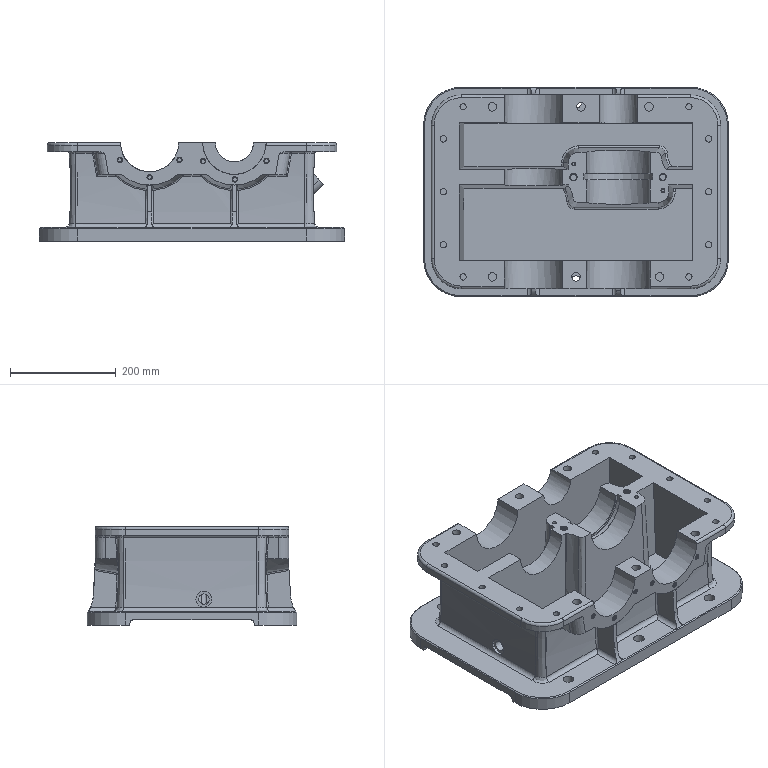Part | NX | features DATUM_CSYS 8, SKETCH 7, EXTRUDE 6, BLEND 2, DATUM_PLANE 2, THREADS 2, BREP 1 | 4 solids | 619 faces | box 576 x 396 x 186 mm | volume 12365991 mm3 | cylinder 377 | plane 119 | spline 80 | cone 19 | torus 16 | sphere 8 | commonest cylinder face diameters 8.5 x250 16 x22 10 x20 6 x16 12 x13 2000 x8